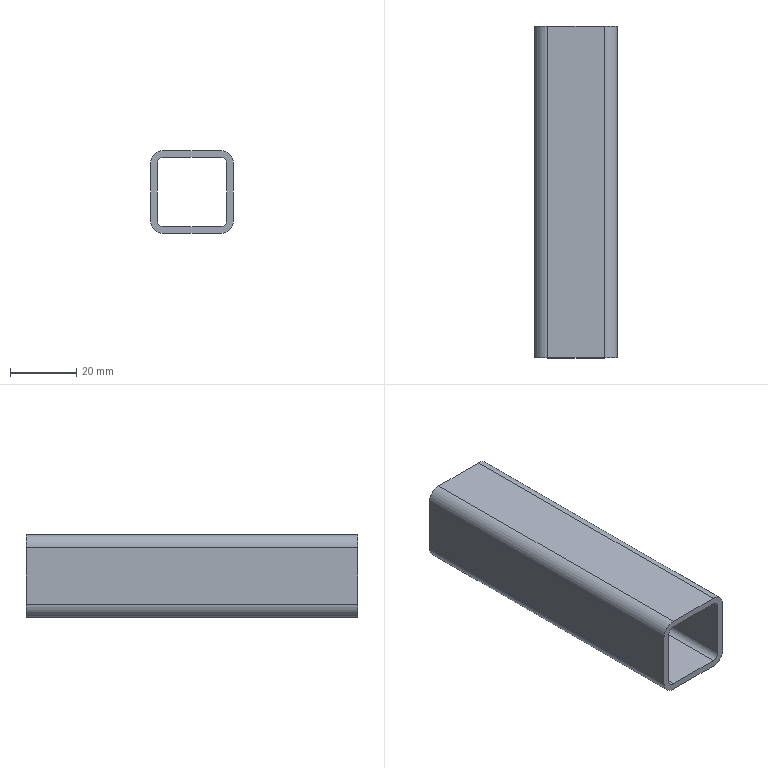Part | SolidWorks | features WeldMemberFeat 1, WeldmentFeature 1 | 1 solid | 18 faces | box 25 x 100 x 25 mm | volume 17370 mm3 | plane 10 | cylinder 8 | commonest cylinder face diameters 4 x4 8 x4
STEP:
#1=CARTESIAN_POINT('',(-12.5,0.,8.5));
#2=VERTEX_POINT('',#1);
#3=CARTESIAN_POINT('',(-8.5,0.,12.5));
#4=VERTEX_POINT('',#3);
#5=CARTESIAN_POINT('',(-8.5,0.,8.5));
#6=DIRECTION('',(0.,1.,0.));
#7=DIRECTION('',(0.,0.,1.));
#8=AXIS2_PLACEMENT_3D('',#5,#6,#7);
#9=CIRCLE('',#8,4.);
#10=EDGE_CURVE('',#2,#4,#9,.T.);
#11=ORIENTED_EDGE('',*,*,#10,.T.);
#12=CARTESIAN_POINT('',(-8.5,100.,12.5));
#13=VERTEX_POINT('',#12);
#14=CARTESIAN_POINT('',(-8.5,100.,12.5));
#15=DIRECTION('',(0.,-1.,0.));
#16=VECTOR('',#15,1000.);
#17=LINE('',#14,#16);
#18=EDGE_CURVE('',#13,#4,#17,.T.);
#19=ORIENTED_EDGE('',*,*,#18,.F.);
#20=CARTESIAN_POINT('',(-12.5,100.,8.5));
#21=VERTEX_POINT('',#20);
#22=CARTESIAN_POINT('',(-8.5,100.,8.5));
#23=DIRECTION('',(0.,1.,0.));
#24=DIRECTION('',(0.,0.,1.));
#25=AXIS2_PLACEMENT_3D('',#22,#23,#24);
#26=CIRCLE('',#25,4.);
#27=EDGE_CURVE('',#21,#13,#26,.T.);
#28=ORIENTED_EDGE('',*,*,#27,.F.);
#29=CARTESIAN_POINT('',(-12.5,100.,8.5));
#30=DIRECTION('',(0.,-1.,0.));
#31=VECTOR('',#30,1000.);
#32=LINE('',#29,#31);
#33=EDGE_CURVE('',#21,#2,#32,.T.);
#34=ORIENTED_EDGE('',*,*,#33,.T.);
#35=EDGE_LOOP('',(#11,#19,#28,#34));
#36=FACE_OUTER_BOUND('',#35,.T.);
#37=CARTESIAN_POINT('',(-8.5,100.,8.5));
#38=DIRECTION('',(0.,-1.,0.));
#39=DIRECTION('',(0.,0.,-1.));
#40=AXIS2_PLACEMENT_3D('',#37,#38,#39);
#41=CYLINDRICAL_SURFACE('',#40,4.);
#42=ADVANCED_FACE('',(#36),#41,.T.);
#43=CARTESIAN_POINT('',(8.5,0.,12.5));
#44=VERTEX_POINT('',#43);
#45=CARTESIAN_POINT('',(-8.5,0.,12.5));
#46=DIRECTION('',(1.,0.,0.));
#47=VECTOR('',#46,1000.);
#48=LINE('',#45,#47);
#49=EDGE_CURVE('',#4,#44,#48,.T.);
#50=ORIENTED_EDGE('',*,*,#49,.T.);
#51=CARTESIAN_POINT('',(8.5,100.,12.5));
#52=VERTEX_POINT('',#51);
#53=CARTESIAN_POINT('',(8.5,100.,12.5));
#54=DIRECTION('',(0.,-1.,0.));
#55=VECTOR('',#54,1000.);
#56=LINE('',#53,#55);
#57=EDGE_CURVE('',#52,#44,#56,.T.);
#58=ORIENTED_EDGE('',*,*,#57,.F.);
#59=CARTESIAN_POINT('',(-8.5,100.,12.5));
#60=DIRECTION('',(1.,0.,0.));
#61=VECTOR('',#60,1000.);
#62=LINE('',#59,#61);
#63=EDGE_CURVE('',#13,#52,#62,.T.);
#64=ORIENTED_EDGE('',*,*,#63,.F.);
#65=ORIENTED_EDGE('',*,*,#18,.T.);
#66=EDGE_LOOP('',(#50,#58,#64,#65));
#67=FACE_OUTER_BOUND('',#66,.T.);
#68=CARTESIAN_POINT('',(-8.5,100.,12.5));
#69=DIRECTION('',(0.,0.,-1.));
#70=DIRECTION('',(-1.,0.,0.));
#71=AXIS2_PLACEMENT_3D('',#68,#69,#70);
#72=PLANE('',#71);
#73=ADVANCED_FACE('',(#67),#72,.F.);
#74=CARTESIAN_POINT('',(12.5,0.,8.5));
#75=VERTEX_POINT('',#74);
#76=CARTESIAN_POINT('',(8.5,0.,8.5));
#77=DIRECTION('',(0.,1.,0.));
#78=DIRECTION('',(0.,0.,1.));
#79=AXIS2_PLACEMENT_3D('',#76,#77,#78);
#80=CIRCLE('',#79,4.);
#81=EDGE_CURVE('',#44,#75,#80,.T.);
#82=ORIENTED_EDGE('',*,*,#81,.T.);
#83=CARTESIAN_POINT('',(12.5,100.,8.5));
#84=VERTEX_POINT('',#83);
#85=CARTESIAN_POINT('',(12.5,100.,8.5));
#86=DIRECTION('',(0.,-1.,0.));
#87=VECTOR('',#86,1000.);
#88=LINE('',#85,#87);
#89=EDGE_CURVE('',#84,#75,#88,.T.);
#90=ORIENTED_EDGE('',*,*,#89,.F.);
#91=CARTESIAN_POINT('',(8.5,100.,8.5));
#92=DIRECTION('',(0.,1.,0.));
#93=DIRECTION('',(0.,0.,1.));
#94=AXIS2_PLACEMENT_3D('',#91,#92,#93);
#95=CIRCLE('',#94,4.);
#96=EDGE_CURVE('',#52,#84,#95,.T.);
#97=ORIENTED_EDGE('',*,*,#96,.F.);
#98=ORIENTED_EDGE('',*,*,#57,.T.);
#99=EDGE_LOOP('',(#82,#90,#97,#98));
#100=FACE_OUTER_BOUND('',#99,.T.);
#101=CARTESIAN_POINT('',(8.5,100.,8.5));
#102=DIRECTION('',(0.,-1.,0.));
#103=DIRECTION('',(0.,0.,-1.));
#104=AXIS2_PLACEMENT_3D('',#101,#102,#103);
#105=CYLINDRICAL_SURFACE('',#104,4.);
#106=ADVANCED_FACE('',(#100),#105,.T.);
#107=CARTESIAN_POINT('',(12.5,0.,-8.5));
#108=VERTEX_POINT('',#107);
#109=CARTESIAN_POINT('',(12.5,0.,-8.5));
#110=DIRECTION('',(0.,0.,-1.));
#111=VECTOR('',#110,1000.);
#112=LINE('',#109,#111);
#113=EDGE_CURVE('',#75,#108,#112,.T.);
#114=ORIENTED_EDGE('',*,*,#113,.T.);
#115=CARTESIAN_POINT('',(12.5,100.,-8.5));
#116=VERTEX_POINT('',#115);
#117=CARTESIAN_POINT('',(12.5,100.,-8.5));
#118=DIRECTION('',(0.,-1.,0.));
#119=VECTOR('',#118,1000.);
#120=LINE('',#117,#119);
#121=EDGE_CURVE('',#116,#108,#120,.T.);
#122=ORIENTED_EDGE('',*,*,#121,.F.);
#123=CARTESIAN_POINT('',(12.5,100.,-8.5));
#124=DIRECTION('',(0.,0.,-1.));
#125=VECTOR('',#124,1000.);
#126=LINE('',#123,#125);
#127=EDGE_CURVE('',#84,#116,#126,.T.);
#128=ORIENTED_EDGE('',*,*,#127,.F.);
#129=ORIENTED_EDGE('',*,*,#89,.T.);
#130=EDGE_LOOP('',(#114,#122,#128,#129));
#131=FACE_OUTER_BOUND('',#130,.T.);
#132=CARTESIAN_POINT('',(12.5,100.,-8.5));
#133=DIRECTION('',(-1.,0.,0.));
#134=DIRECTION('',(0.,0.,1.));
#135=AXIS2_PLACEMENT_3D('',#132,#133,#134);
#136=PLANE('',#135);
#137=ADVANCED_FACE('',(#131),#136,.F.);
#138=CARTESIAN_POINT('',(8.5,0.,-12.5));
#139=VERTEX_POINT('',#138);
#140=CARTESIAN_POINT('',(8.5,0.,-8.5));
#141=DIRECTION('',(0.,1.,0.));
#142=DIRECTION('',(0.,0.,1.));
#143=AXIS2_PLACEMENT_3D('',#140,#141,#142);
#144=CIRCLE('',#143,4.);
#145=EDGE_CURVE('',#108,#139,#144,.T.);
#146=ORIENTED_EDGE('',*,*,#145,.T.);
#147=CARTESIAN_POINT('',(8.5,100.,-12.5));
#148=VERTEX_POINT('',#147);
#149=CARTESIAN_POINT('',(8.5,100.,-12.5));
#150=DIRECTION('',(0.,-1.,0.));
#151=VECTOR('',#150,1000.);
#152=LINE('',#149,#151);
#153=EDGE_CURVE('',#148,#139,#152,.T.);
#154=ORIENTED_EDGE('',*,*,#153,.F.);
#155=CARTESIAN_POINT('',(8.5,100.,-8.5));
#156=DIRECTION('',(0.,1.,0.));
#157=DIRECTION('',(0.,0.,1.));
#158=AXIS2_PLACEMENT_3D('',#155,#156,#157);
#159=CIRCLE('',#158,4.);
#160=EDGE_CURVE('',#116,#148,#159,.T.);
#161=ORIENTED_EDGE('',*,*,#160,.F.);
#162=ORIENTED_EDGE('',*,*,#121,.T.);
#163=EDGE_LOOP('',(#146,#154,#161,#162));
#164=FACE_OUTER_BOUND('',#163,.T.);
#165=CARTESIAN_POINT('',(8.5,100.,-8.5));
#166=DIRECTION('',(0.,-1.,0.));
#167=DIRECTION('',(0.,0.,-1.));
#168=AXIS2_PLACEMENT_3D('',#165,#166,#167);
#169=CYLINDRICAL_SURFACE('',#168,4.);
#170=ADVANCED_FACE('',(#164),#169,.T.);
#171=CARTESIAN_POINT('',(-8.5,0.,-12.5));
#172=VERTEX_POINT('',#171);
#173=CARTESIAN_POINT('',(8.5,0.,-12.5));
#174=DIRECTION('',(-1.,0.,0.));
#175=VECTOR('',#174,1000.);
#176=LINE('',#173,#175);
#177=EDGE_CURVE('',#139,#172,#176,.T.);
#178=ORIENTED_EDGE('',*,*,#177,.T.);
#179=CARTESIAN_POINT('',(-8.5,100.,-12.5));
#180=VERTEX_POINT('',#179);
#181=CARTESIAN_POINT('',(-8.5,100.,-12.5));
#182=DIRECTION('',(0.,-1.,0.));
#183=VECTOR('',#182,1000.);
#184=LINE('',#181,#183);
#185=EDGE_CURVE('',#180,#172,#184,.T.);
#186=ORIENTED_EDGE('',*,*,#185,.F.);
#187=CARTESIAN_POINT('',(8.5,100.,-12.5));
#188=DIRECTION('',(-1.,0.,0.));
#189=VECTOR('',#188,1000.);
#190=LINE('',#187,#189);
#191=EDGE_CURVE('',#148,#180,#190,.T.);
#192=ORIENTED_EDGE('',*,*,#191,.F.);
#193=ORIENTED_EDGE('',*,*,#153,.T.);
#194=EDGE_LOOP('',(#178,#186,#192,#193));
#195=FACE_OUTER_BOUND('',#194,.T.);
#196=CARTESIAN_POINT('',(8.5,100.,-12.5));
#197=DIRECTION('',(0.,0.,1.));
#198=DIRECTION('',(1.,0.,0.));
#199=AXIS2_PLACEMENT_3D('',#196,#197,#198);
#200=PLANE('',#199);
#201=ADVANCED_FACE('',(#195),#200,.F.);
#202=CARTESIAN_POINT('',(-12.5,0.,-8.5));
#203=VERTEX_POINT('',#202);
#204=CARTESIAN_POINT('',(-8.5,0.,-8.5));
#205=DIRECTION('',(0.,1.,0.));
#206=DIRECTION('',(0.,0.,1.));
#207=AXIS2_PLACEMENT_3D('',#204,#205,#206);
#208=CIRCLE('',#207,4.);
#209=EDGE_CURVE('',#172,#203,#208,.T.);
#210=ORIENTED_EDGE('',*,*,#209,.T.);
#211=CARTESIAN_POINT('',(-12.5,100.,-8.5));
#212=VERTEX_POINT('',#211);
#213=CARTESIAN_POINT('',(-12.5,100.,-8.5));
#214=DIRECTION('',(0.,-1.,0.));
#215=VECTOR('',#214,1000.);
#216=LINE('',#213,#215);
#217=EDGE_CURVE('',#212,#203,#216,.T.);
#218=ORIENTED_EDGE('',*,*,#217,.F.);
#219=CARTESIAN_POINT('',(-8.5,100.,-8.5));
#220=DIRECTION('',(0.,1.,0.));
#221=DIRECTION('',(0.,0.,1.));
#222=AXIS2_PLACEMENT_3D('',#219,#220,#221);
#223=CIRCLE('',#222,4.);
#224=EDGE_CURVE('',#180,#212,#223,.T.);
#225=ORIENTED_EDGE('',*,*,#224,.F.);
#226=ORIENTED_EDGE('',*,*,#185,.T.);
#227=EDGE_LOOP('',(#210,#218,#225,#226));
#228=FACE_OUTER_BOUND('',#227,.T.);
#229=CARTESIAN_POINT('',(-8.5,100.,-8.5));
#230=DIRECTION('',(0.,-1.,0.));
#231=DIRECTION('',(0.,0.,-1.));
#232=AXIS2_PLACEMENT_3D('',#229,#230,#231);
#233=CYLINDRICAL_SURFACE('',#232,4.);
#234=ADVANCED_FACE('',(#228),#233,.T.);
#235=CARTESIAN_POINT('',(8.5,0.,10.5));
#236=VERTEX_POINT('',#235);
#237=CARTESIAN_POINT('',(10.5,0.,8.5));
#238=VERTEX_POINT('',#237);
#239=CARTESIAN_POINT('',(8.5,0.,8.5));
#240=DIRECTION('',(0.,1.,0.));
#241=DIRECTION('',(0.,0.,1.));
#242=AXIS2_PLACEMENT_3D('',#239,#240,#241);
#243=CIRCLE('',#242,2.);
#244=EDGE_CURVE('',#236,#238,#243,.T.);
#245=ORIENTED_EDGE('',*,*,#244,.F.);
#246=CARTESIAN_POINT('',(8.5,100.,10.5));
#247=VERTEX_POINT('',#246);
#248=CARTESIAN_POINT('',(8.5,100.,10.5));
#249=DIRECTION('',(0.,-1.,0.));
#250=VECTOR('',#249,1000.);
#251=LINE('',#248,#250);
#252=EDGE_CURVE('',#247,#236,#251,.T.);
#253=ORIENTED_EDGE('',*,*,#252,.F.);
#254=CARTESIAN_POINT('',(10.5,100.,8.5));
#255=VERTEX_POINT('',#254);
#256=CARTESIAN_POINT('',(8.5,100.,8.5));
#257=DIRECTION('',(0.,1.,0.));
#258=DIRECTION('',(0.,0.,1.));
#259=AXIS2_PLACEMENT_3D('',#256,#257,#258);
#260=CIRCLE('',#259,2.);
#261=EDGE_CURVE('',#247,#255,#260,.T.);
#262=ORIENTED_EDGE('',*,*,#261,.T.);
#263=CARTESIAN_POINT('',(10.5,100.,8.5));
#264=DIRECTION('',(0.,-1.,0.));
#265=VECTOR('',#264,1000.);
#266=LINE('',#263,#265);
#267=EDGE_CURVE('',#255,#238,#266,.T.);
#268=ORIENTED_EDGE('',*,*,#267,.T.);
#269=EDGE_LOOP('',(#245,#253,#262,#268));
#270=FACE_OUTER_BOUND('',#269,.T.);
#271=CARTESIAN_POINT('',(8.5,100.,8.5));
#272=DIRECTION('',(0.,-1.,0.));
#273=DIRECTION('',(0.,0.,-1.));
#274=AXIS2_PLACEMENT_3D('',#271,#272,#273);
#275=CYLINDRICAL_SURFACE('',#274,2.);
#276=ADVANCED_FACE('',(#270),#275,.F.);
#277=CARTESIAN_POINT('',(-8.5,0.,10.5));
#278=VERTEX_POINT('',#277);
#279=CARTESIAN_POINT('',(-8.5,0.,10.5));
#280=DIRECTION('',(1.,0.,0.));
#281=VECTOR('',#280,1000.);
#282=LINE('',#279,#281);
#283=EDGE_CURVE('',#278,#236,#282,.T.);
#284=ORIENTED_EDGE('',*,*,#283,.F.);
#285=CARTESIAN_POINT('',(-8.5,100.,10.5));
#286=VERTEX_POINT('',#285);
#287=CARTESIAN_POINT('',(-8.5,100.,10.5));
#288=DIRECTION('',(0.,-1.,0.));
#289=VECTOR('',#288,1000.);
#290=LINE('',#287,#289);
#291=EDGE_CURVE('',#286,#278,#290,.T.);
#292=ORIENTED_EDGE('',*,*,#291,.F.);
#293=CARTESIAN_POINT('',(-8.5,100.,10.5));
#294=DIRECTION('',(1.,0.,0.));
#295=VECTOR('',#294,1000.);
#296=LINE('',#293,#295);
#297=EDGE_CURVE('',#286,#247,#296,.T.);
#298=ORIENTED_EDGE('',*,*,#297,.T.);
#299=ORIENTED_EDGE('',*,*,#252,.T.);
#300=EDGE_LOOP('',(#284,#292,#298,#299));
#301=FACE_OUTER_BOUND('',#300,.T.);
#302=CARTESIAN_POINT('',(-8.5,100.,10.5));
#303=DIRECTION('',(0.,0.,-1.));
#304=DIRECTION('',(-1.,0.,0.));
#305=AXIS2_PLACEMENT_3D('',#302,#303,#304);
#306=PLANE('',#305);
#307=ADVANCED_FACE('',(#301),#306,.T.);
#308=CARTESIAN_POINT('',(-10.5,0.,8.5));
#309=VERTEX_POINT('',#308);
#310=CARTESIAN_POINT('',(-8.5,0.,8.5));
#311=DIRECTION('',(0.,1.,0.));
#312=DIRECTION('',(0.,0.,1.));
#313=AXIS2_PLACEMENT_3D('',#310,#311,#312);
#314=CIRCLE('',#313,2.);
#315=EDGE_CURVE('',#309,#278,#314,.T.);
#316=ORIENTED_EDGE('',*,*,#315,.F.);
#317=CARTESIAN_POINT('',(-10.5,100.,8.5));
#318=VERTEX_POINT('',#317);
#319=CARTESIAN_POINT('',(-10.5,100.,8.5));
#320=DIRECTION('',(0.,-1.,0.));
#321=VECTOR('',#320,1000.);
#322=LINE('',#319,#321);
#323=EDGE_CURVE('',#318,#309,#322,.T.);
#324=ORIENTED_EDGE('',*,*,#323,.F.);
#325=CARTESIAN_POINT('',(-8.5,100.,8.5));
#326=DIRECTION('',(0.,1.,0.));
#327=DIRECTION('',(0.,0.,1.));
#328=AXIS2_PLACEMENT_3D('',#325,#326,#327);
#329=CIRCLE('',#328,2.);
#330=EDGE_CURVE('',#318,#286,#329,.T.);
#331=ORIENTED_EDGE('',*,*,#330,.T.);
#332=ORIENTED_EDGE('',*,*,#291,.T.);
#333=EDGE_LOOP('',(#316,#324,#331,#332));
#334=FACE_OUTER_BOUND('',#333,.T.);
#335=CARTESIAN_POINT('',(-8.5,100.,8.5));
#336=DIRECTION('',(0.,-1.,0.));
#337=DIRECTION('',(0.,0.,-1.));
#338=AXIS2_PLACEMENT_3D('',#335,#336,#337);
#339=CYLINDRICAL_SURFACE('',#338,2.);
#340=ADVANCED_FACE('',(#334),#339,.F.);
#341=CARTESIAN_POINT('',(-10.5,0.,-8.5));
#342=VERTEX_POINT('',#341);
#343=CARTESIAN_POINT('',(-10.5,0.,8.5));
#344=DIRECTION('',(0.,0.,1.));
#345=VECTOR('',#344,1000.);
#346=LINE('',#343,#345);
#347=EDGE_CURVE('',#342,#309,#346,.T.);
#348=ORIENTED_EDGE('',*,*,#347,.F.);
#349=CARTESIAN_POINT('',(-10.5,100.,-8.5));
#350=VERTEX_POINT('',#349);
#351=CARTESIAN_POINT('',(-10.5,100.,-8.5));
#352=DIRECTION('',(0.,-1.,0.));
#353=VECTOR('',#352,1000.);
#354=LINE('',#351,#353);
#355=EDGE_CURVE('',#350,#342,#354,.T.);
#356=ORIENTED_EDGE('',*,*,#355,.F.);
#357=CARTESIAN_POINT('',(-10.5,100.,8.5));
#358=DIRECTION('',(0.,0.,1.));
#359=VECTOR('',#358,1000.);
#360=LINE('',#357,#359);
#361=EDGE_CURVE('',#350,#318,#360,.T.);
#362=ORIENTED_EDGE('',*,*,#361,.T.);
#363=ORIENTED_EDGE('',*,*,#323,.T.);
#364=EDGE_LOOP('',(#348,#356,#362,#363));
#365=FACE_OUTER_BOUND('',#364,.T.);
#366=CARTESIAN_POINT('',(-10.5,100.,8.5));
#367=DIRECTION('',(1.,0.,0.));
#368=DIRECTION('',(0.,0.,-1.));
#369=AXIS2_PLACEMENT_3D('',#366,#367,#368);
#370=PLANE('',#369);
#371=ADVANCED_FACE('',(#365),#370,.T.);
#372=CARTESIAN_POINT('',(-8.5,0.,-10.5));
#373=VERTEX_POINT('',#372);
#374=CARTESIAN_POINT('',(-8.5,0.,-8.5));
#375=DIRECTION('',(0.,1.,0.));
#376=DIRECTION('',(0.,0.,1.));
#377=AXIS2_PLACEMENT_3D('',#374,#375,#376);
#378=CIRCLE('',#377,2.);
#379=EDGE_CURVE('',#373,#342,#378,.T.);
#380=ORIENTED_EDGE('',*,*,#379,.F.);
#381=CARTESIAN_POINT('',(-8.5,100.,-10.5));
#382=VERTEX_POINT('',#381);
#383=CARTESIAN_POINT('',(-8.5,100.,-10.5));
#384=DIRECTION('',(0.,-1.,0.));
#385=VECTOR('',#384,1000.);
#386=LINE('',#383,#385);
#387=EDGE_CURVE('',#382,#373,#386,.T.);
#388=ORIENTED_EDGE('',*,*,#387,.F.);
#389=CARTESIAN_POINT('',(-8.5,100.,-8.5));
#390=DIRECTION('',(0.,1.,0.));
#391=DIRECTION('',(0.,0.,1.));
#392=AXIS2_PLACEMENT_3D('',#389,#390,#391);
#393=CIRCLE('',#392,2.);
#394=EDGE_CURVE('',#382,#350,#393,.T.);
#395=ORIENTED_EDGE('',*,*,#394,.T.);
#396=ORIENTED_EDGE('',*,*,#355,.T.);
#397=EDGE_LOOP('',(#380,#388,#395,#396));
#398=FACE_OUTER_BOUND('',#397,.T.);
#399=CARTESIAN_POINT('',(-8.5,100.,-8.5));
#400=DIRECTION('',(0.,-1.,0.));
#401=DIRECTION('',(0.,0.,-1.));
#402=AXIS2_PLACEMENT_3D('',#399,#400,#401);
#403=CYLINDRICAL_SURFACE('',#402,2.);
#404=ADVANCED_FACE('',(#398),#403,.F.);
#405=CARTESIAN_POINT('',(8.5,0.,-10.5));
#406=VERTEX_POINT('',#405);
#407=CARTESIAN_POINT('',(8.5,0.,-10.5));
#408=DIRECTION('',(-1.,0.,0.));
#409=VECTOR('',#408,1000.);
#410=LINE('',#407,#409);
#411=EDGE_CURVE('',#406,#373,#410,.T.);
#412=ORIENTED_EDGE('',*,*,#411,.F.);
#413=CARTESIAN_POINT('',(8.5,100.,-10.5));
#414=VERTEX_POINT('',#413);
#415=CARTESIAN_POINT('',(8.5,100.,-10.5));
#416=DIRECTION('',(0.,-1.,0.));
#417=VECTOR('',#416,1000.);
#418=LINE('',#415,#417);
#419=EDGE_CURVE('',#414,#406,#418,.T.);
#420=ORIENTED_EDGE('',*,*,#419,.F.);
#421=CARTESIAN_POINT('',(8.5,100.,-10.5));
#422=DIRECTION('',(-1.,0.,0.));
#423=VECTOR('',#422,1000.);
#424=LINE('',#421,#423);
#425=EDGE_CURVE('',#414,#382,#424,.T.);
#426=ORIENTED_EDGE('',*,*,#425,.T.);
#427=ORIENTED_EDGE('',*,*,#387,.T.);
#428=EDGE_LOOP('',(#412,#420,#426,#427));
#429=FACE_OUTER_BOUND('',#428,.T.);
#430=CARTESIAN_POINT('',(8.5,100.,-10.5));
#431=DIRECTION('',(0.,0.,1.));
#432=DIRECTION('',(1.,0.,0.));
#433=AXIS2_PLACEMENT_3D('',#430,#431,#432);
#434=PLANE('',#433);
#435=ADVANCED_FACE('',(#429),#434,.T.);
#436=CARTESIAN_POINT('',(10.5,0.,-8.5));
#437=VERTEX_POINT('',#436);
#438=CARTESIAN_POINT('',(8.5,0.,-8.5));
#439=DIRECTION('',(0.,1.,0.));
#440=DIRECTION('',(0.,0.,1.));
#441=AXIS2_PLACEMENT_3D('',#438,#439,#440);
#442=CIRCLE('',#441,2.);
#443=EDGE_CURVE('',#437,#406,#442,.T.);
#444=ORIENTED_EDGE('',*,*,#443,.F.);
#445=CARTESIAN_POINT('',(10.5,100.,-8.5));
#446=VERTEX_POINT('',#445);
#447=CARTESIAN_POINT('',(10.5,100.,-8.5));
#448=DIRECTION('',(0.,-1.,0.));
#449=VECTOR('',#448,1000.);
#450=LINE('',#447,#449);
#451=EDGE_CURVE('',#446,#437,#450,.T.);
#452=ORIENTED_EDGE('',*,*,#451,.F.);
#453=CARTESIAN_POINT('',(8.5,100.,-8.5));
#454=DIRECTION('',(0.,1.,0.));
#455=DIRECTION('',(0.,0.,1.));
#456=AXIS2_PLACEMENT_3D('',#453,#454,#455);
#457=CIRCLE('',#456,2.);
#458=EDGE_CURVE('',#446,#414,#457,.T.);
#459=ORIENTED_EDGE('',*,*,#458,.T.);
#460=ORIENTED_EDGE('',*,*,#419,.T.);
#461=EDGE_LOOP('',(#444,#452,#459,#460));
#462=FACE_OUTER_BOUND('',#461,.T.);
#463=CARTESIAN_POINT('',(8.5,100.,-8.5));
#464=DIRECTION('',(0.,-1.,0.));
#465=DIRECTION('',(0.,0.,-1.));
#466=AXIS2_PLACEMENT_3D('',#463,#464,#465);
#467=CYLINDRICAL_SURFACE('',#466,2.);
#468=ADVANCED_FACE('',(#462),#467,.F.);
#469=CARTESIAN_POINT('',(10.5,0.,-8.5));
#470=DIRECTION('',(0.,0.,-1.));
#471=VECTOR('',#470,1000.);
#472=LINE('',#469,#471);
#473=EDGE_CURVE('',#238,#437,#472,.T.);
#474=ORIENTED_EDGE('',*,*,#473,.F.);
#475=ORIENTED_EDGE('',*,*,#267,.F.);
#476=CARTESIAN_POINT('',(10.5,100.,-8.5));
#477=DIRECTION('',(0.,0.,-1.));
#478=VECTOR('',#477,1000.);
#479=LINE('',#476,#478);
#480=EDGE_CURVE('',#255,#446,#479,.T.);
#481=ORIENTED_EDGE('',*,*,#480,.T.);
#482=ORIENTED_EDGE('',*,*,#451,.T.);
#483=EDGE_LOOP('',(#474,#475,#481,#482));
#484=FACE_OUTER_BOUND('',#483,.T.);
#485=CARTESIAN_POINT('',(10.5,100.,-8.5));
#486=DIRECTION('',(-1.,0.,0.));
#487=DIRECTION('',(0.,0.,1.));
#488=AXIS2_PLACEMENT_3D('',#485,#486,#487);
#489=PLANE('',#488);
#490=ADVANCED_FACE('',(#484),#489,.T.);
#491=CARTESIAN_POINT('',(-12.5,0.,8.5));
#492=DIRECTION('',(0.,0.,1.));
#493=VECTOR('',#492,1000.);
#494=LINE('',#491,#493);
#495=EDGE_CURVE('',#203,#2,#494,.T.);
#496=ORIENTED_EDGE('',*,*,#495,.T.);
#497=ORIENTED_EDGE('',*,*,#33,.F.);
#498=CARTESIAN_POINT('',(-12.5,100.,8.5));
#499=DIRECTION('',(0.,0.,1.));
#500=VECTOR('',#499,1000.);
#501=LINE('',#498,#500);
#502=EDGE_CURVE('',#212,#21,#501,.T.);
#503=ORIENTED_EDGE('',*,*,#502,.F.);
#504=ORIENTED_EDGE('',*,*,#217,.T.);
#505=EDGE_LOOP('',(#496,#497,#503,#504));
#506=FACE_OUTER_BOUND('',#505,.T.);
#507=CARTESIAN_POINT('',(-12.5,100.,8.5));
#508=DIRECTION('',(1.,0.,0.));
#509=DIRECTION('',(0.,0.,-1.));
#510=AXIS2_PLACEMENT_3D('',#507,#508,#509);
#511=PLANE('',#510);
#512=ADVANCED_FACE('',(#506),#511,.F.);
#513=ORIENTED_EDGE('',*,*,#261,.F.);
#514=ORIENTED_EDGE('',*,*,#297,.F.);
#515=ORIENTED_EDGE('',*,*,#330,.F.);
#516=ORIENTED_EDGE('',*,*,#361,.F.);
#517=ORIENTED_EDGE('',*,*,#394,.F.);
#518=ORIENTED_EDGE('',*,*,#425,.F.);
#519=ORIENTED_EDGE('',*,*,#458,.F.);
#520=ORIENTED_EDGE('',*,*,#480,.F.);
#521=EDGE_LOOP('',(#513,#514,#515,#516,#517,#518,#519,#520));
#522=FACE_BOUND('',#521,.T.);
#523=ORIENTED_EDGE('',*,*,#27,.T.);
#524=ORIENTED_EDGE('',*,*,#63,.T.);
#525=ORIENTED_EDGE('',*,*,#96,.T.);
#526=ORIENTED_EDGE('',*,*,#127,.T.);
#527=ORIENTED_EDGE('',*,*,#160,.T.);
#528=ORIENTED_EDGE('',*,*,#191,.T.);
#529=ORIENTED_EDGE('',*,*,#224,.T.);
#530=ORIENTED_EDGE('',*,*,#502,.T.);
#531=EDGE_LOOP('',(#523,#524,#525,#526,#527,#528,#529,#530));
#532=FACE_OUTER_BOUND('',#531,.T.);
#533=CARTESIAN_POINT('',(-8.5,100.,8.5));
#534=DIRECTION('',(0.,1.,0.));
#535=DIRECTION('',(0.,0.,1.));
#536=AXIS2_PLACEMENT_3D('',#533,#534,#535);
#537=PLANE('',#536);
#538=ADVANCED_FACE('',(#522,#532),#537,.T.);
#539=ORIENTED_EDGE('',*,*,#244,.T.);
#540=ORIENTED_EDGE('',*,*,#473,.T.);
#541=ORIENTED_EDGE('',*,*,#443,.T.);
#542=ORIENTED_EDGE('',*,*,#411,.T.);
#543=ORIENTED_EDGE('',*,*,#379,.T.);
#544=ORIENTED_EDGE('',*,*,#347,.T.);
#545=ORIENTED_EDGE('',*,*,#315,.T.);
#546=ORIENTED_EDGE('',*,*,#283,.T.);
#547=EDGE_LOOP('',(#539,#540,#541,#542,#543,#544,#545,#546));
#548=FACE_BOUND('',#547,.T.);
#549=ORIENTED_EDGE('',*,*,#10,.F.);
#550=ORIENTED_EDGE('',*,*,#495,.F.);
#551=ORIENTED_EDGE('',*,*,#209,.F.);
#552=ORIENTED_EDGE('',*,*,#177,.F.);
#553=ORIENTED_EDGE('',*,*,#145,.F.);
#554=ORIENTED_EDGE('',*,*,#113,.F.);
#555=ORIENTED_EDGE('',*,*,#81,.F.);
#556=ORIENTED_EDGE('',*,*,#49,.F.);
#557=EDGE_LOOP('',(#549,#550,#551,#552,#553,#554,#555,#556));
#558=FACE_OUTER_BOUND('',#557,.T.);
#559=CARTESIAN_POINT('',(-8.5,0.,8.5));
#560=DIRECTION('',(0.,1.,0.));
#561=DIRECTION('',(0.,0.,1.));
#562=AXIS2_PLACEMENT_3D('',#559,#560,#561);
#563=PLANE('',#562);
#564=ADVANCED_FACE('',(#548,#558),#563,.F.);
#565=CLOSED_SHELL('',(#42,#73,#106,#137,#170,#201,#234,#276,#307,#340,#371,#404,#435,#468,#490,#512,#538,#564));
#566=MANIFOLD_SOLID_BREP('',#565);
#567=CARTESIAN_POINT('',(0.,0.,0.));
#568=DIRECTION('',(0.,0.,1.));
#569=DIRECTION('',(1.,0.,0.));
#570=AXIS2_PLACEMENT_3D('',#567,#568,#569);
#571=(LENGTH_UNIT()NAMED_UNIT(*)SI_UNIT(.MILLI.,.METRE.));
#572=UNCERTAINTY_MEASURE_WITH_UNIT(LENGTH_MEASURE(0.00001),#571,'','');
#573=(NAMED_UNIT(*)PLANE_ANGLE_UNIT()SI_UNIT($,.RADIAN.));
#574=(NAMED_UNIT(*)SI_UNIT($,.STERADIAN.)SOLID_ANGLE_UNIT());
#575=(GEOMETRIC_REPRESENTATION_CONTEXT(3)GLOBAL_UNCERTAINTY_ASSIGNED_CONTEXT((#572))GLOBAL_UNIT_ASSIGNED_CONTEXT((#571,#573,#574))REPRESENTATION_CONTEXT('',''));
#576=ADVANCED_BREP_SHAPE_REPRESENTATION('',(#566,#570),#575);